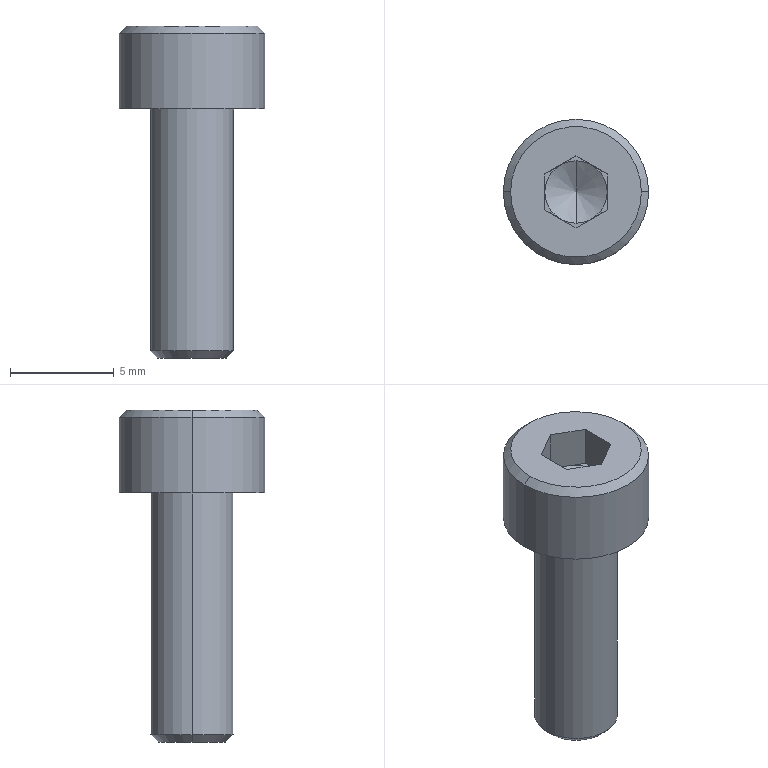Part | SolidWorks | features ICE 2, Chamfer 1, RevCut 1, Revolution 1 | 1 solid | 25 faces | box 7 x 7 x 16 mm | volume 285.079 mm3 | plane 15 | cone 6 | cylinder 4 | commonest cylinder face diameters 4 x2 7 x2
STEP:
#1=CARTESIAN_POINT('',(3.15,0.,4.));
#2=VERTEX_POINT('',#1);
#3=CARTESIAN_POINT('',(-3.15,0.,4.));
#4=VERTEX_POINT('',#3);
#5=CARTESIAN_POINT('',(0.,0.,4.));
#6=DIRECTION('',(0.,0.,1.));
#7=DIRECTION('',(1.,0.,0.));
#8=AXIS2_PLACEMENT_3D('',#5,#6,#7);
#9=CIRCLE('',#8,3.15);
#10=EDGE_CURVE('',#2,#4,#9,.T.);
#11=ORIENTED_EDGE('',*,*,#10,.F.);
#12=CARTESIAN_POINT('',(3.5,0.,3.65));
#13=VERTEX_POINT('',#12);
#14=CARTESIAN_POINT('',(3.15,0.,4.));
#15=DIRECTION('',(0.7071,0.,-0.7071));
#16=VECTOR('',#15,1000.);
#17=LINE('',#14,#16);
#18=EDGE_CURVE('',#2,#13,#17,.T.);
#19=ORIENTED_EDGE('',*,*,#18,.T.);
#20=CARTESIAN_POINT('',(-3.5,0.,3.65));
#21=VERTEX_POINT('',#20);
#22=CARTESIAN_POINT('',(0.,0.,3.65));
#23=DIRECTION('',(0.,0.,-1.));
#24=DIRECTION('',(1.,0.,0.));
#25=AXIS2_PLACEMENT_3D('',#22,#23,#24);
#26=CIRCLE('',#25,3.5);
#27=EDGE_CURVE('',#21,#13,#26,.T.);
#28=ORIENTED_EDGE('',*,*,#27,.F.);
#29=CARTESIAN_POINT('',(-3.15,0.,4.));
#30=DIRECTION('',(-0.7071,0.,-0.7071));
#31=VECTOR('',#30,1000.);
#32=LINE('',#29,#31);
#33=EDGE_CURVE('',#4,#21,#32,.T.);
#34=ORIENTED_EDGE('',*,*,#33,.F.);
#35=EDGE_LOOP('',(#11,#19,#28,#34));
#36=FACE_OUTER_BOUND('',#35,.T.);
#37=CARTESIAN_POINT('',(0.,0.,4.));
#38=DIRECTION('',(0.,0.,-1.));
#39=DIRECTION('',(-1.,0.,0.));
#40=AXIS2_PLACEMENT_3D('',#37,#38,#39);
#41=CONICAL_SURFACE('',#40,3.15,0.7854);
#42=ADVANCED_FACE('',(#36),#41,.T.);
#43=CARTESIAN_POINT('',(-1.65,0.,-12.));
#44=VERTEX_POINT('',#43);
#45=CARTESIAN_POINT('',(1.65,0.,-12.));
#46=VERTEX_POINT('',#45);
#47=CARTESIAN_POINT('',(0.,0.,-12.));
#48=DIRECTION('',(0.,0.,-1.));
#49=DIRECTION('',(-1.,0.,0.));
#50=AXIS2_PLACEMENT_3D('',#47,#48,#49);
#51=CIRCLE('',#50,1.65);
#52=EDGE_CURVE('',#44,#46,#51,.T.);
#53=ORIENTED_EDGE('',*,*,#52,.F.);
#54=CARTESIAN_POINT('',(-2.,0.,-11.65));
#55=VERTEX_POINT('',#54);
#56=CARTESIAN_POINT('',(-1.65,0.,-12.));
#57=DIRECTION('',(-0.7071,0.,0.7071));
#58=VECTOR('',#57,1000.);
#59=LINE('',#56,#58);
#60=EDGE_CURVE('',#44,#55,#59,.T.);
#61=ORIENTED_EDGE('',*,*,#60,.T.);
#62=CARTESIAN_POINT('',(2.,0.,-11.65));
#63=VERTEX_POINT('',#62);
#64=CARTESIAN_POINT('',(0.,0.,-11.65));
#65=DIRECTION('',(0.,0.,1.));
#66=DIRECTION('',(-1.,0.,0.));
#67=AXIS2_PLACEMENT_3D('',#64,#65,#66);
#68=CIRCLE('',#67,2.);
#69=EDGE_CURVE('',#63,#55,#68,.T.);
#70=ORIENTED_EDGE('',*,*,#69,.F.);
#71=CARTESIAN_POINT('',(1.65,0.,-12.));
#72=DIRECTION('',(0.7071,0.,0.7071));
#73=VECTOR('',#72,1000.);
#74=LINE('',#71,#73);
#75=EDGE_CURVE('',#46,#63,#74,.T.);
#76=ORIENTED_EDGE('',*,*,#75,.F.);
#77=EDGE_LOOP('',(#53,#61,#70,#76));
#78=FACE_OUTER_BOUND('',#77,.T.);
#79=CARTESIAN_POINT('',(0.,0.,-12.));
#80=DIRECTION('',(0.,0.,1.));
#81=DIRECTION('',(1.,0.,0.));
#82=AXIS2_PLACEMENT_3D('',#79,#80,#81);
#83=CONICAL_SURFACE('',#82,1.65,0.7854);
#84=ADVANCED_FACE('',(#78),#83,.T.);
#85=CARTESIAN_POINT('',(0.,0.,1.134));
#86=VERTEX_POINT('',#85);
#87=CARTESIAN_POINT('',(0.,-1.5,2.));
#88=VERTEX_POINT('',#87);
#89=CARTESIAN_POINT('',(0.,0.,1.134));
#90=DIRECTION('',(0.,-0.866,0.5));
#91=VECTOR('',#90,1000.);
#92=LINE('',#89,#91);
#93=EDGE_CURVE('',#86,#88,#92,.T.);
#94=ORIENTED_EDGE('',*,*,#93,.F.);
#95=CARTESIAN_POINT('',(0.,1.5,2.));
#96=VERTEX_POINT('',#95);
#97=CARTESIAN_POINT('',(0.,0.,1.134));
#98=DIRECTION('',(0.,0.866,0.5));
#99=VECTOR('',#98,1000.);
#100=LINE('',#97,#99);
#101=EDGE_CURVE('',#86,#96,#100,.T.);
#102=ORIENTED_EDGE('',*,*,#101,.T.);
#103=CARTESIAN_POINT('',(-0.75,1.299,2.));
#104=VERTEX_POINT('',#103);
#105=CARTESIAN_POINT('',(0.,0.,2.));
#106=DIRECTION('',(0.,0.,-1.));
#107=DIRECTION('',(0.,1.,0.));
#108=AXIS2_PLACEMENT_3D('',#105,#106,#107);
#109=CIRCLE('',#108,1.5);
#110=EDGE_CURVE('',#104,#96,#109,.T.);
#111=ORIENTED_EDGE('',*,*,#110,.F.);
#112=CARTESIAN_POINT('',(-1.5,0.,2.));
#113=VERTEX_POINT('',#112);
#114=CARTESIAN_POINT('',(0.,0.,2.));
#115=DIRECTION('',(0.,0.,-1.));
#116=DIRECTION('',(0.,1.,0.));
#117=AXIS2_PLACEMENT_3D('',#114,#115,#116);
#118=CIRCLE('',#117,1.5);
#119=EDGE_CURVE('',#113,#104,#118,.T.);
#120=ORIENTED_EDGE('',*,*,#119,.F.);
#121=CARTESIAN_POINT('',(-0.75,-1.299,2.));
#122=VERTEX_POINT('',#121);
#123=CARTESIAN_POINT('',(0.,0.,2.));
#124=DIRECTION('',(0.,0.,-1.));
#125=DIRECTION('',(0.,1.,0.));
#126=AXIS2_PLACEMENT_3D('',#123,#124,#125);
#127=CIRCLE('',#126,1.5);
#128=EDGE_CURVE('',#122,#113,#127,.T.);
#129=ORIENTED_EDGE('',*,*,#128,.F.);
#130=CARTESIAN_POINT('',(0.,0.,2.));
#131=DIRECTION('',(0.,0.,-1.));
#132=DIRECTION('',(0.,1.,0.));
#133=AXIS2_PLACEMENT_3D('',#130,#131,#132);
#134=CIRCLE('',#133,1.5);
#135=EDGE_CURVE('',#88,#122,#134,.T.);
#136=ORIENTED_EDGE('',*,*,#135,.F.);
#137=EDGE_LOOP('',(#94,#102,#111,#120,#129,#136));
#138=FACE_OUTER_BOUND('',#137,.T.);
#139=CARTESIAN_POINT('',(0.,0.,1001.134));
#140=DIRECTION('',(0.,0.,1.));
#141=DIRECTION('',(0.,-1.,0.));
#142=AXIS2_PLACEMENT_3D('',#139,#140,#141);
#143=CONICAL_SURFACE('',#142,1732.051,1.047);
#144=ADVANCED_FACE('',(#138),#143,.F.);
#145=ORIENTED_EDGE('',*,*,#69,.T.);
#146=CARTESIAN_POINT('',(-2.,0.,0.));
#147=VERTEX_POINT('',#146);
#148=CARTESIAN_POINT('',(-2.,0.,-12.));
#149=DIRECTION('',(0.,0.,1.));
#150=VECTOR('',#149,1000.);
#151=LINE('',#148,#150);
#152=EDGE_CURVE('',#55,#147,#151,.T.);
#153=ORIENTED_EDGE('',*,*,#152,.T.);
#154=CARTESIAN_POINT('',(2.,0.,0.));
#155=VERTEX_POINT('',#154);
#156=CARTESIAN_POINT('',(0.,0.,0.));
#157=DIRECTION('',(0.,0.,-1.));
#158=DIRECTION('',(-1.,0.,0.));
#159=AXIS2_PLACEMENT_3D('',#156,#157,#158);
#160=CIRCLE('',#159,2.);
#161=EDGE_CURVE('',#147,#155,#160,.T.);
#162=ORIENTED_EDGE('',*,*,#161,.T.);
#163=CARTESIAN_POINT('',(2.,0.,-12.));
#164=DIRECTION('',(0.,0.,1.));
#165=VECTOR('',#164,1000.);
#166=LINE('',#163,#165);
#167=EDGE_CURVE('',#63,#155,#166,.T.);
#168=ORIENTED_EDGE('',*,*,#167,.F.);
#169=EDGE_LOOP('',(#145,#153,#162,#168));
#170=FACE_OUTER_BOUND('',#169,.T.);
#171=CARTESIAN_POINT('',(0.,0.,-12.));
#172=DIRECTION('',(0.,0.,1.));
#173=DIRECTION('',(1.,0.,0.));
#174=AXIS2_PLACEMENT_3D('',#171,#172,#173);
#175=CYLINDRICAL_SURFACE('',#174,2.);
#176=ADVANCED_FACE('',(#170),#175,.T.);
#177=CARTESIAN_POINT('',(3.5,0.,0.));
#178=VERTEX_POINT('',#177);
#179=CARTESIAN_POINT('',(-3.5,0.,0.));
#180=VERTEX_POINT('',#179);
#181=CARTESIAN_POINT('',(0.,0.,0.));
#182=DIRECTION('',(0.,0.,1.));
#183=DIRECTION('',(1.,0.,0.));
#184=AXIS2_PLACEMENT_3D('',#181,#182,#183);
#185=CIRCLE('',#184,3.5);
#186=EDGE_CURVE('',#178,#180,#185,.T.);
#187=ORIENTED_EDGE('',*,*,#186,.T.);
#188=CARTESIAN_POINT('',(-3.5,0.,0.));
#189=DIRECTION('',(0.,0.,1.));
#190=VECTOR('',#189,1000.);
#191=LINE('',#188,#190);
#192=EDGE_CURVE('',#180,#21,#191,.T.);
#193=ORIENTED_EDGE('',*,*,#192,.T.);
#194=ORIENTED_EDGE('',*,*,#27,.T.);
#195=CARTESIAN_POINT('',(3.5,0.,0.));
#196=DIRECTION('',(0.,0.,1.));
#197=VECTOR('',#196,1000.);
#198=LINE('',#195,#197);
#199=EDGE_CURVE('',#178,#13,#198,.T.);
#200=ORIENTED_EDGE('',*,*,#199,.F.);
#201=EDGE_LOOP('',(#187,#193,#194,#200));
#202=FACE_OUTER_BOUND('',#201,.T.);
#203=CARTESIAN_POINT('',(0.,0.,0.));
#204=DIRECTION('',(0.,0.,1.));
#205=DIRECTION('',(1.,0.,0.));
#206=AXIS2_PLACEMENT_3D('',#203,#204,#205);
#207=CYLINDRICAL_SURFACE('',#206,3.5);
#208=ADVANCED_FACE('',(#202),#207,.T.);
#209=CARTESIAN_POINT('',(1.5,0.866,2.));
#210=VERTEX_POINT('',#209);
#211=CARTESIAN_POINT('',(0.75,1.299,2.));
#212=VERTEX_POINT('',#211);
#213=CARTESIAN_POINT('',(1.5,0.866,2.));
#214=DIRECTION('',(-0.866,0.5,0.));
#215=VECTOR('',#214,1000.);
#216=LINE('',#213,#215);
#217=EDGE_CURVE('',#210,#212,#216,.T.);
#218=ORIENTED_EDGE('',*,*,#217,.T.);
#219=CARTESIAN_POINT('',(1.5,0.,2.));
#220=VERTEX_POINT('',#219);
#221=CARTESIAN_POINT('',(0.,0.,2.));
#222=DIRECTION('',(0.,0.,-1.));
#223=DIRECTION('',(0.,1.,0.));
#224=AXIS2_PLACEMENT_3D('',#221,#222,#223);
#225=CIRCLE('',#224,1.5);
#226=EDGE_CURVE('',#212,#220,#225,.T.);
#227=ORIENTED_EDGE('',*,*,#226,.T.);
#228=CARTESIAN_POINT('',(1.5,-0.866,2.));
#229=DIRECTION('',(0.,1.,0.));
#230=VECTOR('',#229,1000.);
#231=LINE('',#228,#230);
#232=EDGE_CURVE('',#220,#210,#231,.T.);
#233=ORIENTED_EDGE('',*,*,#232,.T.);
#234=EDGE_LOOP('',(#218,#227,#233));
#235=FACE_OUTER_BOUND('',#234,.T.);
#236=CARTESIAN_POINT('',(0.,0.,2.));
#237=DIRECTION('',(0.,0.,1.));
#238=DIRECTION('',(1.,0.,0.));
#239=AXIS2_PLACEMENT_3D('',#236,#237,#238);
#240=PLANE('',#239);
#241=ADVANCED_FACE('',(#235),#240,.T.);
#242=CARTESIAN_POINT('',(1.5,-0.866,2.));
#243=VERTEX_POINT('',#242);
#244=CARTESIAN_POINT('',(1.5,-0.866,2.));
#245=DIRECTION('',(0.,1.,0.));
#246=VECTOR('',#245,1000.);
#247=LINE('',#244,#246);
#248=EDGE_CURVE('',#243,#220,#247,.T.);
#249=ORIENTED_EDGE('',*,*,#248,.T.);
#250=CARTESIAN_POINT('',(0.75,-1.299,2.));
#251=VERTEX_POINT('',#250);
#252=CARTESIAN_POINT('',(0.,0.,2.));
#253=DIRECTION('',(0.,0.,-1.));
#254=DIRECTION('',(0.,1.,0.));
#255=AXIS2_PLACEMENT_3D('',#252,#253,#254);
#256=CIRCLE('',#255,1.5);
#257=EDGE_CURVE('',#220,#251,#256,.T.);
#258=ORIENTED_EDGE('',*,*,#257,.T.);
#259=CARTESIAN_POINT('',(0.,-1.732,2.));
#260=DIRECTION('',(0.866,0.5,0.));
#261=VECTOR('',#260,1000.);
#262=LINE('',#259,#261);
#263=EDGE_CURVE('',#251,#243,#262,.T.);
#264=ORIENTED_EDGE('',*,*,#263,.T.);
#265=EDGE_LOOP('',(#249,#258,#264));
#266=FACE_OUTER_BOUND('',#265,.T.);
#267=CARTESIAN_POINT('',(0.,0.,2.));
#268=DIRECTION('',(0.,0.,1.));
#269=DIRECTION('',(1.,0.,0.));
#270=AXIS2_PLACEMENT_3D('',#267,#268,#269);
#271=PLANE('',#270);
#272=ADVANCED_FACE('',(#266),#271,.T.);
#273=CARTESIAN_POINT('',(0.,-1.732,2.));
#274=VERTEX_POINT('',#273);
#275=CARTESIAN_POINT('',(0.,-1.732,2.));
#276=DIRECTION('',(0.866,0.5,0.));
#277=VECTOR('',#276,1000.);
#278=LINE('',#275,#277);
#279=EDGE_CURVE('',#274,#251,#278,.T.);
#280=ORIENTED_EDGE('',*,*,#279,.T.);
#281=CARTESIAN_POINT('',(0.,0.,2.));
#282=DIRECTION('',(0.,0.,-1.));
#283=DIRECTION('',(0.,1.,0.));
#284=AXIS2_PLACEMENT_3D('',#281,#282,#283);
#285=CIRCLE('',#284,1.5);
#286=EDGE_CURVE('',#251,#88,#285,.T.);
#287=ORIENTED_EDGE('',*,*,#286,.T.);
#288=ORIENTED_EDGE('',*,*,#135,.T.);
#289=CARTESIAN_POINT('',(-1.5,-0.866,2.));
#290=DIRECTION('',(0.866,-0.5,0.));
#291=VECTOR('',#290,1000.);
#292=LINE('',#289,#291);
#293=EDGE_CURVE('',#122,#274,#292,.T.);
#294=ORIENTED_EDGE('',*,*,#293,.T.);
#295=EDGE_LOOP('',(#280,#287,#288,#294));
#296=FACE_OUTER_BOUND('',#295,.T.);
#297=CARTESIAN_POINT('',(0.,0.,2.));
#298=DIRECTION('',(0.,0.,1.));
#299=DIRECTION('',(1.,0.,0.));
#300=AXIS2_PLACEMENT_3D('',#297,#298,#299);
#301=PLANE('',#300);
#302=ADVANCED_FACE('',(#296),#301,.T.);
#303=CARTESIAN_POINT('',(-1.5,-0.866,2.));
#304=VERTEX_POINT('',#303);
#305=CARTESIAN_POINT('',(-1.5,-0.866,2.));
#306=DIRECTION('',(0.866,-0.5,0.));
#307=VECTOR('',#306,1000.);
#308=LINE('',#305,#307);
#309=EDGE_CURVE('',#304,#122,#308,.T.);
#310=ORIENTED_EDGE('',*,*,#309,.T.);
#311=ORIENTED_EDGE('',*,*,#128,.T.);
#312=CARTESIAN_POINT('',(-1.5,0.866,2.));
#313=DIRECTION('',(0.,-1.,0.));
#314=VECTOR('',#313,1000.);
#315=LINE('',#312,#314);
#316=EDGE_CURVE('',#113,#304,#315,.T.);
#317=ORIENTED_EDGE('',*,*,#316,.T.);
#318=EDGE_LOOP('',(#310,#311,#317));
#319=FACE_OUTER_BOUND('',#318,.T.);
#320=CARTESIAN_POINT('',(0.,0.,2.));
#321=DIRECTION('',(0.,0.,1.));
#322=DIRECTION('',(1.,0.,0.));
#323=AXIS2_PLACEMENT_3D('',#320,#321,#322);
#324=PLANE('',#323);
#325=ADVANCED_FACE('',(#319),#324,.T.);
#326=CARTESIAN_POINT('',(-1.5,0.866,2.));
#327=VERTEX_POINT('',#326);
#328=CARTESIAN_POINT('',(-1.5,0.866,2.));
#329=DIRECTION('',(0.,-1.,0.));
#330=VECTOR('',#329,1000.);
#331=LINE('',#328,#330);
#332=EDGE_CURVE('',#327,#113,#331,.T.);
#333=ORIENTED_EDGE('',*,*,#332,.T.);
#334=ORIENTED_EDGE('',*,*,#119,.T.);
#335=CARTESIAN_POINT('',(0.,1.732,2.));
#336=DIRECTION('',(-0.866,-0.5,0.));
#337=VECTOR('',#336,1000.);
#338=LINE('',#335,#337);
#339=EDGE_CURVE('',#104,#327,#338,.T.);
#340=ORIENTED_EDGE('',*,*,#339,.T.);
#341=EDGE_LOOP('',(#333,#334,#340));
#342=FACE_OUTER_BOUND('',#341,.T.);
#343=CARTESIAN_POINT('',(0.,0.,2.));
#344=DIRECTION('',(0.,0.,1.));
#345=DIRECTION('',(1.,0.,0.));
#346=AXIS2_PLACEMENT_3D('',#343,#344,#345);
#347=PLANE('',#346);
#348=ADVANCED_FACE('',(#342),#347,.T.);
#349=CARTESIAN_POINT('',(0.,1.732,2.));
#350=VERTEX_POINT('',#349);
#351=CARTESIAN_POINT('',(0.,1.732,2.));
#352=DIRECTION('',(-0.866,-0.5,0.));
#353=VECTOR('',#352,1000.);
#354=LINE('',#351,#353);
#355=EDGE_CURVE('',#350,#104,#354,.T.);
#356=ORIENTED_EDGE('',*,*,#355,.T.);
#357=ORIENTED_EDGE('',*,*,#110,.T.);
#358=CARTESIAN_POINT('',(0.,0.,2.));
#359=DIRECTION('',(0.,0.,-1.));
#360=DIRECTION('',(0.,1.,0.));
#361=AXIS2_PLACEMENT_3D('',#358,#359,#360);
#362=CIRCLE('',#361,1.5);
#363=EDGE_CURVE('',#96,#212,#362,.T.);
#364=ORIENTED_EDGE('',*,*,#363,.T.);
#365=CARTESIAN_POINT('',(1.5,0.866,2.));
#366=DIRECTION('',(-0.866,0.5,0.));
#367=VECTOR('',#366,1000.);
#368=LINE('',#365,#367);
#369=EDGE_CURVE('',#212,#350,#368,.T.);
#370=ORIENTED_EDGE('',*,*,#369,.T.);
#371=EDGE_LOOP('',(#356,#357,#364,#370));
#372=FACE_OUTER_BOUND('',#371,.T.);
#373=CARTESIAN_POINT('',(0.,0.,2.));
#374=DIRECTION('',(0.,0.,1.));
#375=DIRECTION('',(1.,0.,0.));
#376=AXIS2_PLACEMENT_3D('',#373,#374,#375);
#377=PLANE('',#376);
#378=ADVANCED_FACE('',(#372),#377,.T.);
#379=ORIENTED_EDGE('',*,*,#186,.F.);
#380=CARTESIAN_POINT('',(0.,0.,0.));
#381=DIRECTION('',(0.,0.,1.));
#382=DIRECTION('',(1.,0.,0.));
#383=AXIS2_PLACEMENT_3D('',#380,#381,#382);
#384=CIRCLE('',#383,3.5);
#385=EDGE_CURVE('',#180,#178,#384,.T.);
#386=ORIENTED_EDGE('',*,*,#385,.F.);
#387=EDGE_LOOP('',(#379,#386));
#388=FACE_OUTER_BOUND('',#387,.T.);
#389=CARTESIAN_POINT('',(0.,0.,0.));
#390=DIRECTION('',(0.,0.,-1.));
#391=DIRECTION('',(-1.,0.,0.));
#392=AXIS2_PLACEMENT_3D('',#389,#390,#391);
#393=CIRCLE('',#392,2.);
#394=EDGE_CURVE('',#155,#147,#393,.T.);
#395=ORIENTED_EDGE('',*,*,#394,.F.);
#396=ORIENTED_EDGE('',*,*,#161,.F.);
#397=EDGE_LOOP('',(#395,#396));
#398=FACE_BOUND('',#397,.T.);
#399=CARTESIAN_POINT('',(3.5,0.,0.));
#400=DIRECTION('',(0.,0.,-1.));
#401=DIRECTION('',(-1.,0.,0.));
#402=AXIS2_PLACEMENT_3D('',#399,#400,#401);
#403=PLANE('',#402);
#404=ADVANCED_FACE('',(#388,#398),#403,.T.);
#405=ORIENTED_EDGE('',*,*,#192,.F.);
#406=ORIENTED_EDGE('',*,*,#385,.T.);
#407=ORIENTED_EDGE('',*,*,#199,.T.);
#408=CARTESIAN_POINT('',(0.,0.,3.65));
#409=DIRECTION('',(0.,0.,-1.));
#410=DIRECTION('',(1.,0.,0.));
#411=AXIS2_PLACEMENT_3D('',#408,#409,#410);
#412=CIRCLE('',#411,3.5);
#413=EDGE_CURVE('',#13,#21,#412,.T.);
#414=ORIENTED_EDGE('',*,*,#413,.T.);
#415=EDGE_LOOP('',(#405,#406,#407,#414));
#416=FACE_OUTER_BOUND('',#415,.T.);
#417=CARTESIAN_POINT('',(0.,0.,0.));
#418=DIRECTION('',(0.,0.,1.));
#419=DIRECTION('',(1.,0.,0.));
#420=AXIS2_PLACEMENT_3D('',#417,#418,#419);
#421=CYLINDRICAL_SURFACE('',#420,3.5);
#422=ADVANCED_FACE('',(#416),#421,.T.);
#423=CARTESIAN_POINT('',(0.,0.,4.));
#424=DIRECTION('',(0.,0.,1.));
#425=DIRECTION('',(1.,0.,0.));
#426=AXIS2_PLACEMENT_3D('',#423,#424,#425);
#427=CIRCLE('',#426,3.15);
#428=EDGE_CURVE('',#4,#2,#427,.T.);
#429=ORIENTED_EDGE('',*,*,#428,.T.);
#430=ORIENTED_EDGE('',*,*,#10,.T.);
#431=EDGE_LOOP('',(#429,#430));
#432=FACE_OUTER_BOUND('',#431,.T.);
#433=CARTESIAN_POINT('',(0.,-1.732,4.));
#434=VERTEX_POINT('',#433);
#435=CARTESIAN_POINT('',(1.5,-0.866,4.));
#436=VERTEX_POINT('',#435);
#437=CARTESIAN_POINT('',(0.,-1.732,4.));
#438=DIRECTION('',(0.866,0.5,0.));
#439=VECTOR('',#438,1000.);
#440=LINE('',#437,#439);
#441=EDGE_CURVE('',#434,#436,#440,.T.);
#442=ORIENTED_EDGE('',*,*,#441,.F.);
#443=CARTESIAN_POINT('',(-1.5,-0.866,4.));
#444=VERTEX_POINT('',#443);
#445=CARTESIAN_POINT('',(-1.5,-0.866,4.));
#446=DIRECTION('',(0.866,-0.5,0.));
#447=VECTOR('',#446,1000.);
#448=LINE('',#445,#447);
#449=EDGE_CURVE('',#444,#434,#448,.T.);
#450=ORIENTED_EDGE('',*,*,#449,.F.);
#451=CARTESIAN_POINT('',(-1.5,0.866,4.));
#452=VERTEX_POINT('',#451);
#453=CARTESIAN_POINT('',(-1.5,0.866,4.));
#454=DIRECTION('',(0.,-1.,0.));
#455=VECTOR('',#454,1000.);
#456=LINE('',#453,#455);
#457=EDGE_CURVE('',#452,#444,#456,.T.);
#458=ORIENTED_EDGE('',*,*,#457,.F.);
#459=CARTESIAN_POINT('',(0.,1.732,4.));
#460=VERTEX_POINT('',#459);
#461=CARTESIAN_POINT('',(0.,1.732,4.));
#462=DIRECTION('',(-0.866,-0.5,0.));
#463=VECTOR('',#462,1000.);
#464=LINE('',#461,#463);
#465=EDGE_CURVE('',#460,#452,#464,.T.);
#466=ORIENTED_EDGE('',*,*,#465,.F.);
#467=CARTESIAN_POINT('',(1.5,0.866,4.));
#468=VERTEX_POINT('',#467);
#469=CARTESIAN_POINT('',(1.5,0.866,4.));
#470=DIRECTION('',(-0.866,0.5,0.));
#471=VECTOR('',#470,1000.);
#472=LINE('',#469,#471);
#473=EDGE_CURVE('',#468,#460,#472,.T.);
#474=ORIENTED_EDGE('',*,*,#473,.F.);
#475=CARTESIAN_POINT('',(1.5,-0.866,4.));
#476=DIRECTION('',(0.,1.,0.));
#477=VECTOR('',#476,1000.);
#478=LINE('',#475,#477);
#479=EDGE_CURVE('',#436,#468,#478,.T.);
#480=ORIENTED_EDGE('',*,*,#479,.F.);
#481=EDGE_LOOP('',(#442,#450,#458,#466,#474,#480));
#482=FACE_BOUND('',#481,.T.);
#483=CARTESIAN_POINT('',(0.,0.,4.));
#484=DIRECTION('',(0.,0.,1.));
#485=DIRECTION('',(1.,0.,0.));
#486=AXIS2_PLACEMENT_3D('',#483,#484,#485);
#487=PLANE('',#486);
#488=ADVANCED_FACE('',(#432,#482),#487,.T.);
#489=ORIENTED_EDGE('',*,*,#152,.F.);
#490=CARTESIAN_POINT('',(0.,0.,-11.65));
#491=DIRECTION('',(0.,0.,1.));
#492=DIRECTION('',(-1.,0.,0.));
#493=AXIS2_PLACEMENT_3D('',#490,#491,#492);
#494=CIRCLE('',#493,2.);
#495=EDGE_CURVE('',#55,#63,#494,.T.);
#496=ORIENTED_EDGE('',*,*,#495,.T.);
#497=ORIENTED_EDGE('',*,*,#167,.T.);
#498=ORIENTED_EDGE('',*,*,#394,.T.);
#499=EDGE_LOOP('',(#489,#496,#497,#498));
#500=FACE_OUTER_BOUND('',#499,.T.);
#501=CARTESIAN_POINT('',(0.,0.,-12.));
#502=DIRECTION('',(0.,0.,1.));
#503=DIRECTION('',(1.,0.,0.));
#504=AXIS2_PLACEMENT_3D('',#501,#502,#503);
#505=CYLINDRICAL_SURFACE('',#504,2.);
#506=ADVANCED_FACE('',(#500),#505,.T.);
#507=CARTESIAN_POINT('',(0.,0.,-12.));
#508=DIRECTION('',(0.,0.,-1.));
#509=DIRECTION('',(-1.,0.,0.));
#510=AXIS2_PLACEMENT_3D('',#507,#508,#509);
#511=CIRCLE('',#510,1.65);
#512=EDGE_CURVE('',#46,#44,#511,.T.);
#513=ORIENTED_EDGE('',*,*,#512,.T.);
#514=ORIENTED_EDGE('',*,*,#52,.T.);
#515=EDGE_LOOP('',(#513,#514));
#516=FACE_OUTER_BOUND('',#515,.T.);
#517=CARTESIAN_POINT('',(0.,0.,-12.));
#518=DIRECTION('',(0.,0.,-1.));
#519=DIRECTION('',(-1.,0.,0.));
#520=AXIS2_PLACEMENT_3D('',#517,#518,#519);
#521=PLANE('',#520);
#522=ADVANCED_FACE('',(#516),#521,.T.);
#523=ORIENTED_EDGE('',*,*,#441,.T.);
#524=CARTESIAN_POINT('',(1.5,-0.866,2.));
#525=DIRECTION('',(0.,0.,1.));
#526=VECTOR('',#525,1000.);
#527=LINE('',#524,#526);
#528=EDGE_CURVE('',#243,#436,#527,.T.);
#529=ORIENTED_EDGE('',*,*,#528,.F.);
#530=ORIENTED_EDGE('',*,*,#263,.F.);
#531=ORIENTED_EDGE('',*,*,#279,.F.);
#532=CARTESIAN_POINT('',(0.,-1.732,2.));
#533=DIRECTION('',(0.,0.,1.));
#534=VECTOR('',#533,1000.);
#535=LINE('',#532,#534);
#536=EDGE_CURVE('',#274,#434,#535,.T.);
#537=ORIENTED_EDGE('',*,*,#536,.T.);
#538=EDGE_LOOP('',(#523,#529,#530,#531,#537));
#539=FACE_OUTER_BOUND('',#538,.T.);
#540=CARTESIAN_POINT('',(0.,-1.732,2.));
#541=DIRECTION('',(0.5,-0.866,0.));
#542=DIRECTION('',(0.866,0.5,0.));
#543=AXIS2_PLACEMENT_3D('',#540,#541,#542);
#544=PLANE('',#543);
#545=ADVANCED_FACE('',(#539),#544,.F.);
#546=ORIENTED_EDGE('',*,*,#449,.T.);
#547=ORIENTED_EDGE('',*,*,#536,.F.);
#548=ORIENTED_EDGE('',*,*,#293,.F.);
#549=ORIENTED_EDGE('',*,*,#309,.F.);
#550=CARTESIAN_POINT('',(-1.5,-0.866,2.));
#551=DIRECTION('',(0.,0.,1.));
#552=VECTOR('',#551,1000.);
#553=LINE('',#550,#552);
#554=EDGE_CURVE('',#304,#444,#553,.T.);
#555=ORIENTED_EDGE('',*,*,#554,.T.);
#556=EDGE_LOOP('',(#546,#547,#548,#549,#555));
#557=FACE_OUTER_BOUND('',#556,.T.);
#558=CARTESIAN_POINT('',(-1.5,-0.866,2.));
#559=DIRECTION('',(-0.5,-0.866,0.));
#560=DIRECTION('',(0.866,-0.5,0.));
#561=AXIS2_PLACEMENT_3D('',#558,#559,#560);
#562=PLANE('',#561);
#563=ADVANCED_FACE('',(#557),#562,.F.);
#564=ORIENTED_EDGE('',*,*,#457,.T.);
#565=ORIENTED_EDGE('',*,*,#554,.F.);
#566=ORIENTED_EDGE('',*,*,#316,.F.);
#567=ORIENTED_EDGE('',*,*,#332,.F.);
#568=CARTESIAN_POINT('',(-1.5,0.866,2.));
#569=DIRECTION('',(0.,0.,1.));
#570=VECTOR('',#569,1000.);
#571=LINE('',#568,#570);
#572=EDGE_CURVE('',#327,#452,#571,.T.);
#573=ORIENTED_EDGE('',*,*,#572,.T.);
#574=EDGE_LOOP('',(#564,#565,#566,#567,#573));
#575=FACE_OUTER_BOUND('',#574,.T.);
#576=CARTESIAN_POINT('',(-1.5,0.866,2.));
#577=DIRECTION('',(-1.,0.,0.));
#578=DIRECTION('',(0.,-1.,0.));
#579=AXIS2_PLACEMENT_3D('',#576,#577,#578);
#580=PLANE('',#579);
#581=ADVANCED_FACE('',(#575),#580,.F.);
#582=ORIENTED_EDGE('',*,*,#465,.T.);
#583=ORIENTED_EDGE('',*,*,#572,.F.);
#584=ORIENTED_EDGE('',*,*,#339,.F.);
#585=ORIENTED_EDGE('',*,*,#355,.F.);
#586=CARTESIAN_POINT('',(0.,1.732,2.));
#587=DIRECTION('',(0.,0.,1.));
#588=VECTOR('',#587,1000.);
#589=LINE('',#586,#588);
#590=EDGE_CURVE('',#350,#460,#589,.T.);
#591=ORIENTED_EDGE('',*,*,#590,.T.);
#592=EDGE_LOOP('',(#582,#583,#584,#585,#591));
#593=FACE_OUTER_BOUND('',#592,.T.);
#594=CARTESIAN_POINT('',(0.,1.732,2.));
#595=DIRECTION('',(-0.5,0.866,0.));
#596=DIRECTION('',(-0.866,-0.5,0.));
#597=AXIS2_PLACEMENT_3D('',#594,#595,#596);
#598=PLANE('',#597);
#599=ADVANCED_FACE('',(#593),#598,.F.);
#600=ORIENTED_EDGE('',*,*,#473,.T.);
#601=ORIENTED_EDGE('',*,*,#590,.F.);
#602=ORIENTED_EDGE('',*,*,#369,.F.);
#603=ORIENTED_EDGE('',*,*,#217,.F.);
#604=CARTESIAN_POINT('',(1.5,0.866,2.));
#605=DIRECTION('',(0.,0.,1.));
#606=VECTOR('',#605,1000.);
#607=LINE('',#604,#606);
#608=EDGE_CURVE('',#210,#468,#607,.T.);
#609=ORIENTED_EDGE('',*,*,#608,.T.);
#610=EDGE_LOOP('',(#600,#601,#602,#603,#609));
#611=FACE_OUTER_BOUND('',#610,.T.);
#612=CARTESIAN_POINT('',(1.5,0.866,2.));
#613=DIRECTION('',(0.5,0.866,0.));
#614=DIRECTION('',(-0.866,0.5,0.));
#615=AXIS2_PLACEMENT_3D('',#612,#613,#614);
#616=PLANE('',#615);
#617=ADVANCED_FACE('',(#611),#616,.F.);
#618=ORIENTED_EDGE('',*,*,#479,.T.);
#619=ORIENTED_EDGE('',*,*,#608,.F.);
#620=ORIENTED_EDGE('',*,*,#232,.F.);
#621=ORIENTED_EDGE('',*,*,#248,.F.);
#622=ORIENTED_EDGE('',*,*,#528,.T.);
#623=EDGE_LOOP('',(#618,#619,#620,#621,#622));
#624=FACE_OUTER_BOUND('',#623,.T.);
#625=CARTESIAN_POINT('',(1.5,-0.866,2.));
#626=DIRECTION('',(1.,0.,0.));
#627=DIRECTION('',(0.,1.,0.));
#628=AXIS2_PLACEMENT_3D('',#625,#626,#627);
#629=PLANE('',#628);
#630=ADVANCED_FACE('',(#624),#629,.F.);
#631=ORIENTED_EDGE('',*,*,#101,.F.);
#632=ORIENTED_EDGE('',*,*,#93,.T.);
#633=ORIENTED_EDGE('',*,*,#286,.F.);
#634=ORIENTED_EDGE('',*,*,#257,.F.);
#635=ORIENTED_EDGE('',*,*,#226,.F.);
#636=ORIENTED_EDGE('',*,*,#363,.F.);
#637=EDGE_LOOP('',(#631,#632,#633,#634,#635,#636));
#638=FACE_OUTER_BOUND('',#637,.T.);
#639=CARTESIAN_POINT('',(0.,0.,1001.134));
#640=DIRECTION('',(0.,0.,1.));
#641=DIRECTION('',(0.,-1.,0.));
#642=AXIS2_PLACEMENT_3D('',#639,#640,#641);
#643=CONICAL_SURFACE('',#642,1732.051,1.047);
#644=ADVANCED_FACE('',(#638),#643,.F.);
#645=ORIENTED_EDGE('',*,*,#60,.F.);
#646=ORIENTED_EDGE('',*,*,#512,.F.);
#647=ORIENTED_EDGE('',*,*,#75,.T.);
#648=ORIENTED_EDGE('',*,*,#495,.F.);
#649=EDGE_LOOP('',(#645,#646,#647,#648));
#650=FACE_OUTER_BOUND('',#649,.T.);
#651=CARTESIAN_POINT('',(0.,0.,-12.));
#652=DIRECTION('',(0.,0.,1.));
#653=DIRECTION('',(1.,0.,0.));
#654=AXIS2_PLACEMENT_3D('',#651,#652,#653);
#655=CONICAL_SURFACE('',#654,1.65,0.7854);
#656=ADVANCED_FACE('',(#650),#655,.T.);
#657=ORIENTED_EDGE('',*,*,#18,.F.);
#658=ORIENTED_EDGE('',*,*,#428,.F.);
#659=ORIENTED_EDGE('',*,*,#33,.T.);
#660=ORIENTED_EDGE('',*,*,#413,.F.);
#661=EDGE_LOOP('',(#657,#658,#659,#660));
#662=FACE_OUTER_BOUND('',#661,.T.);
#663=CARTESIAN_POINT('',(0.,0.,4.));
#664=DIRECTION('',(0.,0.,-1.));
#665=DIRECTION('',(-1.,0.,0.));
#666=AXIS2_PLACEMENT_3D('',#663,#664,#665);
#667=CONICAL_SURFACE('',#666,3.15,0.7854);
#668=ADVANCED_FACE('',(#662),#667,.T.);
#669=CLOSED_SHELL('',(#42,#84,#144,#176,#208,#241,#272,#302,#325,#348,#378,#404,#422,#488,#506,#522,#545,#563,#581,#599,#617,#630,#644,#656,#668));
#670=MANIFOLD_SOLID_BREP('',#669);
#671=CARTESIAN_POINT('',(0.,0.,0.));
#672=DIRECTION('',(0.,0.,1.));
#673=DIRECTION('',(1.,0.,0.));
#674=AXIS2_PLACEMENT_3D('',#671,#672,#673);
#675=(LENGTH_UNIT()NAMED_UNIT(*)SI_UNIT(.MILLI.,.METRE.));
#676=UNCERTAINTY_MEASURE_WITH_UNIT(LENGTH_MEASURE(0.00001),#675,'','');
#677=(NAMED_UNIT(*)PLANE_ANGLE_UNIT()SI_UNIT($,.RADIAN.));
#678=(NAMED_UNIT(*)SI_UNIT($,.STERADIAN.)SOLID_ANGLE_UNIT());
#679=(GEOMETRIC_REPRESENTATION_CONTEXT(3)GLOBAL_UNCERTAINTY_ASSIGNED_CONTEXT((#676))GLOBAL_UNIT_ASSIGNED_CONTEXT((#675,#677,#678))REPRESENTATION_CONTEXT('',''));
#680=ADVANCED_BREP_SHAPE_REPRESENTATION('',(#670,#674),#679);